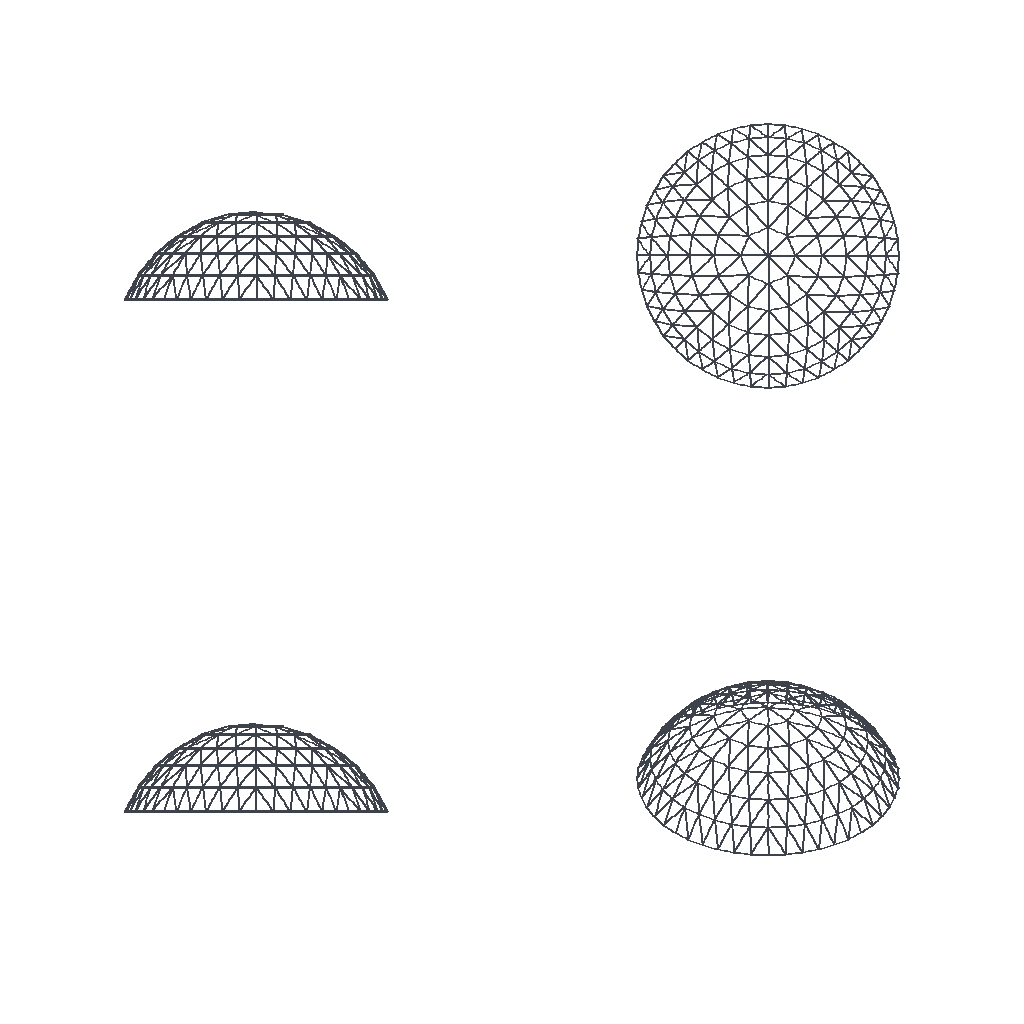Simulation study | abaqus
Set-up summary:
category,name,step,type,value,unit,region
solver,abaqus
solver,version,,,Abaqus/Standard 2020
units,not stated in the deck,,not stated
analysis,deck,,transient,transient
load_step,Step-1,Step-1,transient
load_step,Step-2,Step-2,transient
load_step,requested,,,2
mesh,nodes,,,3297
mesh,elements,,,3584
element_type,T3D2,,truss,3584
load,load commands in deck,,count,6
bc,support commands in deck,,count,1
material,MATERIAL-1,,in results
check,setup vs results,,match,"per instance, exact: element labels, types and connectivity; labels of the nodes the elements use; coordinates of those nodes at SINGLE_PRECISION in 1 of 1 instance(s)"
Abaqus input file, long lists of numbers shortened:
*Heading
** Job name: Job-1 Model name: Model-1
** Generated by: Abaqus/CAE 2020
*Preprint, echo=NO, model=NO, history=NO, contact=NO
**
** PARTS
**
*Part, name=part
*Node
      1,   154697.453,   6174.262, 0.0002526
      2,   157307.984,   6345.365, 0.0002526
** (3295 more lines like these left out)
*Element, type=T3D2
1,   1, 170
2, 170, 171
** (3582 more lines like these left out)
*Nset, nset=Set-1, generate
    1,  3297,     1
*Elset, elset=Set-1, generate
    1,  3584,     1
** Section: Section-1
*Solid Section, elset=Set-1, material=Material-1
0.0115,
*End Part
**
**
** ASSEMBLY
**
*Assembly, name=Assembly
**
*Instance, name=part-1, part=part
-154697.458, -26174.262,      -13333.
*End Instance
**
*Nset, nset=Set-1, instance=part-1
    1,    2,    6,    8,    9,   10,   11,   13,   14,   36,   37,   43,   44,   46,   47,   56
   80,   83,  103,  104,  106,  107,  111,  112,  113,  128,  129,  130,  132,  133,  134,  135
** (13 more lines like these left out)
*Elset, elset=Set-1, instance=part-1
    1,    2,    3,    4,    5,   61,   62,   63,   64,   65,   66,   67,   68,   69,   70,   71
   72,   73,   74,   75,   76,   77,   78,   79,   80,   99,  100,  101,  102,  103,  281,  282
** (13 more lines like these left out)
*Nset, nset=Set-2, instance=part-1
    3,    4,    5,    7,   12,   15,   16,   17,   18,   19,   20,   21,   22,   23,   24,   25
   26,   27,   28,   29,   30,   31,   32,   33,   34,   35,   38,   39,   40,   41,   42,   45
** (145 more lines like these left out)
*Elset, elset=Set-2, instance=part-1
   16,   17,   18,   19,   20,   21,   22,   23,   24,   25,   26,   27,   46,   47,   48,   49
   50,   51,  114,  115,  116,  117,  118,  119,  120,  121,  122,  123,  124,  125,  126,  127
** (157 more lines like these left out)
*End Assembly
*Amplitude, name=Amp-4, definition=PERIODIC
1,             10.,              0.,              0.
            6.5,              0.
*Amplitude, name=horizon
           0.01,       0.2817,            0.02,       0.281,           0.022,       0.2811,           0.025,        0.2813
          0.029,       0.2817,            0.03,       0.2818,           0.032,       0.2821,           0.035,       0.2824
          0.036,       0.2826,            0.04,       0.2832,           0.042,       0.2836,           0.044,        0.284
          0.045,       0.2842,           0.046,       0.2844,           0.048,       0.2848,            0.05,       0.285
          0.055,       0.2859,            0.06,       0.3122,           0.065,       0.3359,           0.067,       0.3345
           0.07,       0.3366,           0.075,       0.3762,            0.08,       0.4346,           0.085,       0.4502
           0.09,       0.4789,           0.095,       0.5231,             0.1,        0.5791,            0.11,       0.5499
           0.12,         0.6681,            0.13,       0.8193,           0.133,       0.8078,            0.14,       0.7421
           0.15,       0.649,            0.16,       0.5537,            0.17,       0.7679,            0.18,       0.7256
           0.19,       0.6464,             0.2,       0.6249,            0.22,       0.6911,            0.24,       0.7918
           0.25,       0.813,            0.26,       0.8004,            0.28,       0.7195,            0.29,       0.6802
            0.3,        0.6517,            0.32,       0.6672,            0.34,       0.5925,            0.35,       0.5908
           0.36,       0.6594,            0.38,       0.6755,             0.4,       0.612,            0.42,       0.5694
           0.44,       0.7364,            0.45,       0.8089,            0.46,       0.8388,            0.48,       0.7868
            0.5,       0.7376,            0.55,       0.7345,             0.6,       0.5393,            0.65,       0.491
          0.667,       0.5055,             0.7,       0.5563,            0.75,       0.437,             0.8,       0.5056
           0.85,       0.5637,             0.9,       0.4935,            0.95,        0.4995,              1.,       0.4698
            1.1,       0.3752,             1.2,       0.3289,             1.3,       0.2714,             1.4,       0.196
            1.5,       0.1595,             1.6,       0.1643,             1.7,       0.1808,             1.8,       0.1936
            1.9,       0.1993,              2.,       0.1975,             2.2,       0.193,             2.4,       0.1705
            2.5,        0.1549,             2.6,       0.1391,             2.8,       0.1257,              3.,       0.1045
            3.2,      0.07918,             3.4,      0.06694,             3.5,       0.06223,             3.6,      0.05767
            3.8,      0.04918,              4.,      0.04174,             4.2,      0.03537,             4.4,      0.02999
            4.6,      0.02551,             4.8,      0.02178,              5.,      0.0187,             5.5,      0.01451
             6.,      0.01194,             6.5,      0.01029,              7.,      0.00799,             7.5,      0.006708
             8.,      0.005695,             8.5,      0.004886,              9.,      0.004232,             9.5,       0.003698
            10.,        0.003256,             11.,      0.002646,             12.,      0.002231,             13.,      0.001907
            14.,      0.001648,             15.,      0.001438,             20.,      0.0008133
*Amplitude, name=horizon2
           0.01,       0.2118,            0.02,       0.2108,           0.022,       0.2109,           0.025,       0.2111
          0.029,       0.2114,            0.03,       0.2114,           0.032,       0.2116,           0.035,       0.2119
          0.036,       0.212,            0.04,       0.2127,           0.042,       0.213,           0.044,       0.2133
          0.045,       0.2136,           0.046,       0.2139,           0.048,       0.214,            0.05,       0.214
          0.055,        0.2159,            0.06,       0.215,           0.065,       0.2175,           0.067,       0.2197
           0.07,       0.2236,           0.075,       0.2276,            0.08,       0.2448,           0.085,        0.2651
           0.09,       0.283,           0.095,       0.3048,             0.1,       0.3106,            0.11,       0.3392
           0.12,       0.3157,            0.13,       0.3533,           0.133,       0.3916,            0.14,       0.3567
           0.15,       0.4043,            0.16,       0.4423,            0.17,        0.3959,            0.18,       0.469
           0.19,        0.5035,             0.2,       0.5121,            0.22,       0.5809,            0.24,       0.4775
           0.25,       0.5404,            0.26,       0.4936,            0.28,       0.4208,            0.29,       0.4125
            0.3,       0.4326,            0.32,       0.4539,            0.34,       0.3988,            0.35,       0.4202
           0.36,       0.4476,            0.38,       0.4846,             0.4,        0.5712,            0.42,       0.5051
           0.44,       0.4904,            0.45,        0.4921,            0.46,       0.491,            0.48,       0.4804
            0.5,       0.5175,            0.55,       0.5566,             0.6,       0.5719,            0.65,       0.4516
          0.667,       0.4218,             0.7,       0.4303,            0.75,       0.4336,             0.8,       0.4367
           0.85,       0.3404,             0.9,       0.3427,            0.95,       0.2871,              1.,       0.2786
            1.1,       0.2679,             1.2,       0.3451,             1.3,       0.291,             1.4,       0.2104
            1.5,       0.1903,             1.6,       0.1859,             1.7,       0.1826,             1.8,       0.1816
            1.9,       0.2005,              2.,       0.2277,             2.2,         0.1782,             2.4,       0.1355
            2.5,         0.1224,             2.6,       0.1194,             2.8,       0.1132,              3.,        0.1081
            3.2,      0.09402,             3.4,      0.08227,             3.5,      0.07823,             3.6,      0.07433
            3.8,      0.06691,              4.,      0.06014,             4.2,      0.05412,             4.4,      0.04862
            4.6,      0.04637,             4.8,      0.04983,              5.,      0.05694,             5.5,      0.05427
             6.,      0.04511,             6.5,      0.03527,              7.,      0.03161,             7.5,      0.02689
             8.,      0.02316,             8.5,      0.01927,              9.,      0.01566,             9.5,       0.01251
            10.,      0.009856,             11.,      0.008477,             12.,      0.006416,             13.,      0.005234
            14.,      0.004521,             15.,      0.003978,             20.,      0.002307
*Amplitude, name=vertical
           0.01,           0.181,            0.02,           0.178,           0.022,           0.179,           0.025,           0.181
          0.029,           0.184,            0.03,           0.185,           0.032,           0.186,           0.035,           0.188
          0.036,           0.189,            0.04,           0.192,           0.042,           0.194,           0.044,           0.195
          0.045,           0.196,           0.046,           0.197,           0.048,           0.199,            0.05,           0.201
          0.055,           0.203,            0.06,           0.204,           0.065,           0.237,           0.067,           0.256
           0.07,           0.267,           0.075,           0.297,            0.08,           0.297,           0.085,           0.383
           0.09,           0.442,           0.095,           0.445,             0.1,           0.515,            0.11,           0.609
           0.12,           0.686,            0.13,           0.394,           0.133,            0.35,            0.14,           0.324
           0.15,           0.315,            0.16,           0.273,            0.17,           0.224,            0.18,           0.213
           0.19,           0.214,             0.2,           0.226,            0.22,           0.258,            0.24,           0.257
           0.25,           0.274,            0.26,           0.291,            0.28,           0.264,            0.29,           0.236
            0.3,           0.213,            0.32,            0.19,            0.34,           0.198,            0.35,             0.2
           0.36,           0.198,            0.38,           0.187,             0.4,           0.186,            0.42,           0.176
           0.44,           0.148,            0.45,           0.132,            0.46,           0.126,            0.48,           0.118
            0.5,           0.135,            0.55,           0.173,             0.6,           0.174,            0.65,           0.149
          0.667,           0.135,             0.7,           0.107,            0.75,          0.0895,             0.8,          0.0882
           0.85,           0.084,             0.9,          0.0807,            0.95,          0.0784,              1.,           0.061
            1.1,          0.0473,             1.2,          0.0542,             1.3,          0.0577,             1.4,          0.0405
            1.5,          0.0454,             1.6,          0.0414,             1.7,          0.0464,             1.8,          0.0456
            1.9,          0.0388,              2.,          0.0391,             2.2,          0.0307,             2.4,          0.0269
            2.5,          0.0302,             2.6,          0.0318,             2.8,          0.0279,              3.,          0.0278
            3.2,          0.0235,             3.4,           0.021,             3.5,            0.02,             3.6,          0.0189
            3.8,          0.0188,              4.,          0.0177,             4.2,          0.0168,             4.4,          0.0158
            4.6,          0.0133,             4.8,          0.0119,              5.,          0.0106,             5.5,         0.00783
             6.,         0.00635,             6.5,         0.00477,              7.,         0.00345,             7.5,         0.00288
             8.,         0.00248,             8.5,         0.00215,              9.,         0.00188,             9.5,         0.00166
            10.,         0.00147,             11.,         0.00117,             12.,        0.000957,             13.,        0.000795
            14.,        0.000671,             15.,        0.000573,             20.,        0.000302
**
** MATERIALS
**
*Material, name=Material-1
*Density
7890.,
*Elastic
 2.1e+11, 0.3
*Plastic
 2.35e+08,0.
** ----------------------------------------------------------------
**
** STEP: Step-1
**
*Step, name=Step-1, nlgeom=YES, inc=10000
*Dynamic
0.002,4.,2e-05
**
** BOUNDARY CONDITIONS
**
** Name: BC-1 Type: 对称/反对称/完全固定
*Boundary
Set-1, PINNED
**
** LOADS
**
** Name: Load-1   Type: Gravity
*Dload, op=NEW, amplitude=Amp-4
Set-2, GRAV, 0.1, 1., 0., 0.
** Name: Load-2   Type: Gravity
*Dload, op=NEW, amplitude=Amp-4
Set-2, GRAV, 0.1, 0., 1., 0.
** Name: Load-3   Type: Gravity
*Dload, op=NEW, amplitude=Amp-4
Set-2, GRAV, 0.1, 0., 0., 1.
**
** OUTPUT REQUESTS
**
*Restart, write, frequency=0
**
** FIELD OUTPUT: F-Output-1
**
*Output, field, variable=PRESELECT, time interval=0.05
**
** HISTORY OUTPUT: H-Output-1
**
*Output, history, variable=PRESELECT, frequency=1
*End Step
** ----------------------------------------------------------------
**
** STEP: Step-2
**
*Step, name=Step-2, nlgeom=YES, inc=1000
*Dynamic
0.01,6.,6e-05
**
** LOADS
**
** Name: Load-1   Type: Gravity
*Dload, op=NEW, amplitude=Amp-4
Set-2, GRAV, 1., 1., 0., 0.
** Name: Load-2   Type: Gravity
*Dload, op=NEW, amplitude=Amp-4
Set-2, GRAV, 1., 0., 1., 0.
** Name: Load-3   Type: Gravity
*Dload, op=NEW, amplitude=Amp-4
Set-2, GRAV, 1., 0., 0., 1.
**
** OUTPUT REQUESTS
**
*Restart, write, frequency=0
**
** FIELD OUTPUT: F-Output-1
**
*Output, field, variable=PRESELECT, frequency=1
**
** HISTORY OUTPUT: H-Output-1
**
*Output, history, variable=PRESELECT, frequency=1
*End Step
Results summary:
result,step,,completed,increments=170 time=4.0/4.0
result,step,,completed,increments=107 time=6.0/6.0
result,analysis,,,transient
result,last_loadstep,,,2
result,primary field,,,U
result,reaction total,,FX,-1401217.091,model units
result,reaction total,,FY,-1401320.927,model units
result,reaction total,,FZ,-12851093.473,model units